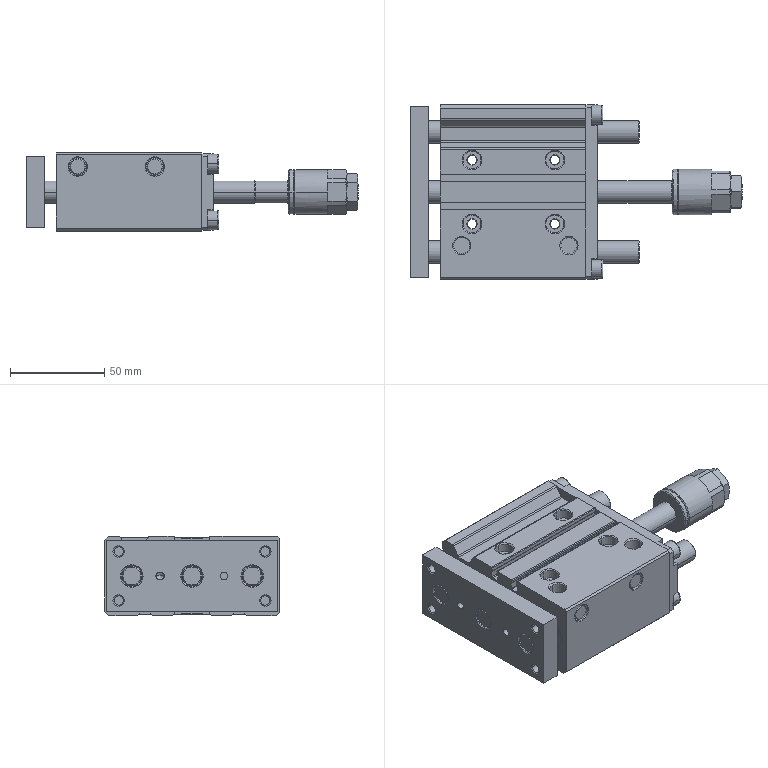Part | SolidWorks | features BaseBody 3, MoveFace 1 | 3 solids | 534 faces | box 176.5 x 93 x 42 mm | volume 329147 mm3 | cylinder 203 | plane 183 | cone 136 | spline 12 | commonest cylinder face diameters 0.8 x28 4.917 x24 4 x21 12 x14 0.4 x12 10 x10